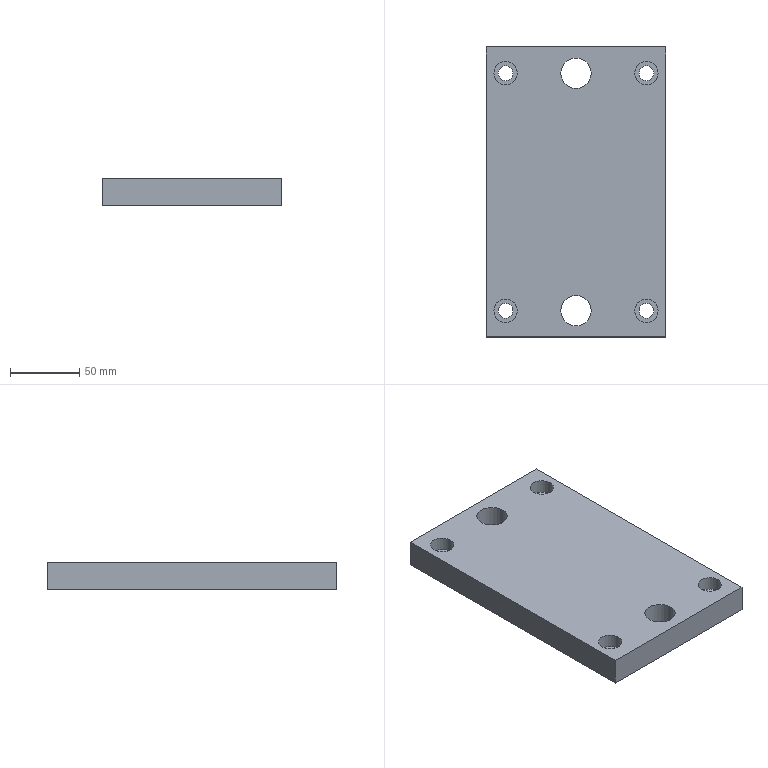Part | STEP file | YBQDJ-YB-28 | 1 solid | 20 faces | box 130 x 210 x 20 mm | volume 518119 mm3 | cylinder 10 | plane 10 | commonest cylinder face diameters 10.7 x4 17 x4 22 x2